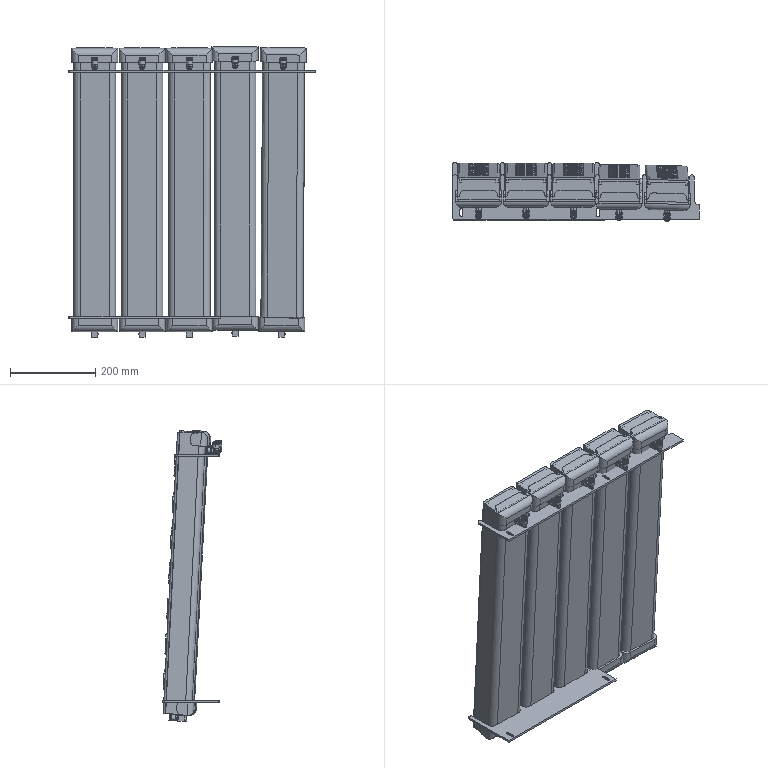Part | SolidWorks | 122 solids | 7172 faces | volume 7857189 mm3 | plane 3961 | cylinder 2196 | cone 630 | torus 200 | spline 135 | sphere 50 | commonest cylinder face diameters 10.222 x280 30.787 x280 8.17 x140 6.779 x120 30 x100 7.866 x95